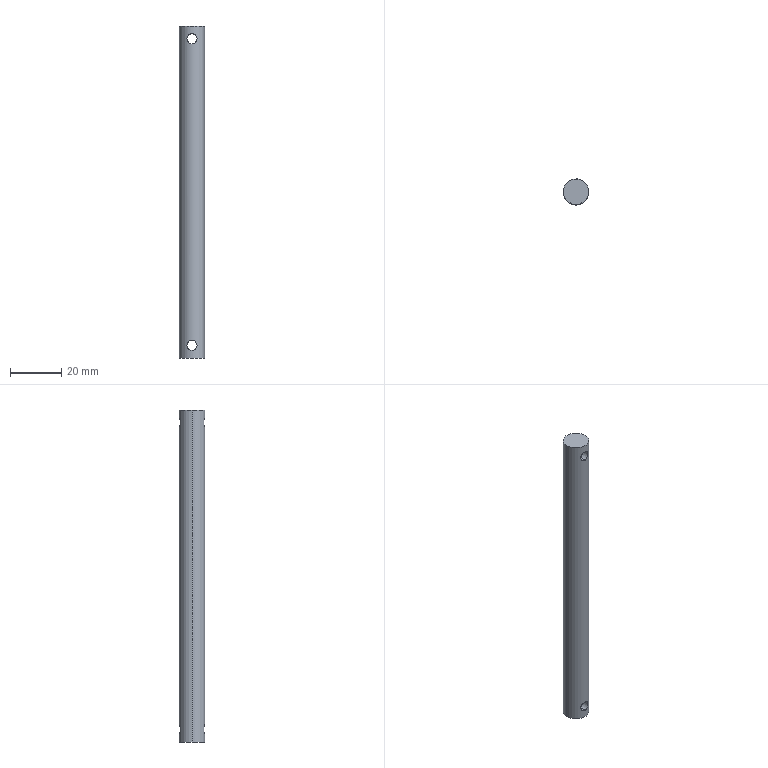Part | SolidWorks | features Extrusion 1, ICE 1 | 1 solid | 8 faces | box 10 x 10 x 130 mm | volume 9964 mm3 | cylinder 6 | plane 2 | commonest cylinder face diameters 4 x4 10 x2
STEP:
#1=CARTESIAN_POINT('',(0.,-5.,58.));
#2=VERTEX_POINT('',#1);
#3=CARTESIAN_POINT('',(0.,-5.,62.));
#4=VERTEX_POINT('',#3);
#5=CARTESIAN_POINT('',(0.,-5.,58.));
#6=CARTESIAN_POINT('',(-0.1316,-5.,58.));
#7=CARTESIAN_POINT('',(-0.2649,-4.995,58.013));
#8=CARTESIAN_POINT('',(-0.5241,-4.974,58.065));
#9=CARTESIAN_POINT('',(-0.6493,-4.959,58.104));
#10=CARTESIAN_POINT('',(-0.8912,-4.921,58.205));
#11=CARTESIAN_POINT('',(-1.008,-4.899,58.268));
#12=CARTESIAN_POINT('',(-1.223,-4.849,58.412));
#13=CARTESIAN_POINT('',(-1.323,-4.823,58.495));
#14=CARTESIAN_POINT('',(-1.507,-4.768,58.679));
#15=CARTESIAN_POINT('',(-1.589,-4.741,58.779));
#16=CARTESIAN_POINT('',(-1.733,-4.691,58.994));
#17=CARTESIAN_POINT('',(-1.796,-4.667,59.11));
#18=CARTESIAN_POINT('',(-1.896,-4.627,59.351));
#19=CARTESIAN_POINT('',(-1.935,-4.611,59.476));
#20=CARTESIAN_POINT('',(-1.987,-4.589,59.734));
#21=CARTESIAN_POINT('',(-2.,-4.583,59.868));
#22=CARTESIAN_POINT('',(-2.,-4.583,60.263));
#23=CARTESIAN_POINT('',(-1.946,-4.607,60.529));
#24=CARTESIAN_POINT('',(-1.796,-4.667,60.89));
#25=CARTESIAN_POINT('',(-1.733,-4.691,61.006));
#26=CARTESIAN_POINT('',(-1.589,-4.742,61.222));
#27=CARTESIAN_POINT('',(-1.507,-4.769,61.322));
#28=CARTESIAN_POINT('',(-1.323,-4.823,61.505));
#29=CARTESIAN_POINT('',(-1.222,-4.85,61.589));
#30=CARTESIAN_POINT('',(-1.007,-4.899,61.733));
#31=CARTESIAN_POINT('',(-0.8926,-4.921,61.795));
#32=CARTESIAN_POINT('',(-0.5273,-4.978,61.947));
#33=CARTESIAN_POINT('',(-0.2671,-5.,62.));
#34=CARTESIAN_POINT('',(0.,-5.,62.));
#35=B_SPLINE_CURVE_WITH_KNOTS('',3,(#5,#6,#7,#8,#9,#10,#11,#12,#13,#14,#15,#16,#17,#18,#19,#20,#21,#22,#23,#24,#25,#26,#27,#28,#29,#30,#31,#32,#33,#34),.UNSPECIFIED.,.F.,.F.,(4,2,2,2,2,2,2,2,2,2,2,2,2,2,4),(0.00632,0.006715,0.007109,0.007504,0.007899,0.008293,0.008688,0.009083,0.009478,0.01027,0.01066,0.01106,0.01145,0.01185,0.01264),.UNSPECIFIED.);
#36=EDGE_CURVE('',#2,#4,#35,.T.);
#37=ORIENTED_EDGE('',*,*,#36,.F.);
#38=CARTESIAN_POINT('',(0.,5.,58.));
#39=VERTEX_POINT('',#38);
#40=CARTESIAN_POINT('',(0.,-5.,58.));
#41=DIRECTION('',(0.,1.,0.));
#42=VECTOR('',#41,1000.);
#43=LINE('',#40,#42);
#44=EDGE_CURVE('',#2,#39,#43,.T.);
#45=ORIENTED_EDGE('',*,*,#44,.T.);
#46=CARTESIAN_POINT('',(0.,5.,62.));
#47=VERTEX_POINT('',#46);
#48=CARTESIAN_POINT('',(0.,5.,62.));
#49=CARTESIAN_POINT('',(-0.1337,5.,62.));
#50=CARTESIAN_POINT('',(-0.2648,4.995,61.987));
#51=CARTESIAN_POINT('',(-0.5224,4.974,61.935));
#52=CARTESIAN_POINT('',(-0.6502,4.959,61.896));
#53=CARTESIAN_POINT('',(-0.8919,4.921,61.795));
#54=CARTESIAN_POINT('',(-1.006,4.899,61.733));
#55=CARTESIAN_POINT('',(-1.223,4.849,61.588));
#56=CARTESIAN_POINT('',(-1.324,4.822,61.505));
#57=CARTESIAN_POINT('',(-1.597,4.742,61.231));
#58=CARTESIAN_POINT('',(-1.746,4.687,61.01));
#59=CARTESIAN_POINT('',(-1.896,4.627,60.65));
#60=CARTESIAN_POINT('',(-1.935,4.61,60.523));
#61=CARTESIAN_POINT('',(-1.987,4.588,60.264));
#62=CARTESIAN_POINT('',(-2.,4.583,60.133));
#63=CARTESIAN_POINT('',(-2.,4.583,59.869));
#64=CARTESIAN_POINT('',(-1.987,4.588,59.735));
#65=CARTESIAN_POINT('',(-1.935,4.611,59.477));
#66=CARTESIAN_POINT('',(-1.897,4.627,59.352));
#67=CARTESIAN_POINT('',(-1.795,4.667,59.108));
#68=CARTESIAN_POINT('',(-1.733,4.691,58.994));
#69=CARTESIAN_POINT('',(-1.589,4.741,58.778));
#70=CARTESIAN_POINT('',(-1.505,4.769,58.677));
#71=CARTESIAN_POINT('',(-1.322,4.823,58.494));
#72=CARTESIAN_POINT('',(-1.223,4.85,58.412));
#73=CARTESIAN_POINT('',(-1.006,4.899,58.267));
#74=CARTESIAN_POINT('',(-0.8898,4.922,58.204));
#75=CARTESIAN_POINT('',(-0.5291,4.978,58.054));
#76=CARTESIAN_POINT('',(-0.2633,5.,58.));
#77=CARTESIAN_POINT('',(0.,5.,58.));
#78=B_SPLINE_CURVE_WITH_KNOTS('',3,(#48,#49,#50,#51,#52,#53,#54,#55,#56,#57,#58,#59,#60,#61,#62,#63,#64,#65,#66,#67,#68,#69,#70,#71,#72,#73,#74,#75,#76,#77),.UNSPECIFIED.,.F.,.F.,(4,2,2,2,2,2,2,2,2,2,2,2,2,2,4),(0.,0.000395,0.00079,0.001185,0.00158,0.00237,0.002765,0.00316,0.003555,0.00395,0.004345,0.00474,0.005135,0.00553,0.00632),.UNSPECIFIED.);
#79=EDGE_CURVE('',#47,#39,#78,.T.);
#80=ORIENTED_EDGE('',*,*,#79,.F.);
#81=CARTESIAN_POINT('',(0.,-5.,62.));
#82=DIRECTION('',(0.,1.,0.));
#83=VECTOR('',#82,1000.);
#84=LINE('',#81,#83);
#85=EDGE_CURVE('',#4,#47,#84,.T.);
#86=ORIENTED_EDGE('',*,*,#85,.F.);
#87=EDGE_LOOP('',(#37,#45,#80,#86));
#88=FACE_OUTER_BOUND('',#87,.T.);
#89=CARTESIAN_POINT('',(0.,-5.,60.));
#90=DIRECTION('',(0.,1.,0.));
#91=DIRECTION('',(0.,0.,1.));
#92=AXIS2_PLACEMENT_3D('',#89,#90,#91);
#93=CYLINDRICAL_SURFACE('',#92,2.);
#94=ADVANCED_FACE('',(#88),#93,.F.);
#95=CARTESIAN_POINT('',(0.,-5.,-62.));
#96=VERTEX_POINT('',#95);
#97=CARTESIAN_POINT('',(0.,-5.,-58.));
#98=VERTEX_POINT('',#97);
#99=CARTESIAN_POINT('',(0.,-5.,-62.));
#100=CARTESIAN_POINT('',(-0.1316,-5.,-62.));
#101=CARTESIAN_POINT('',(-0.2649,-4.995,-61.987));
#102=CARTESIAN_POINT('',(-0.5241,-4.974,-61.935));
#103=CARTESIAN_POINT('',(-0.6493,-4.959,-61.896));
#104=CARTESIAN_POINT('',(-0.8912,-4.921,-61.795));
#105=CARTESIAN_POINT('',(-1.008,-4.899,-61.732));
#106=CARTESIAN_POINT('',(-1.223,-4.849,-61.588));
#107=CARTESIAN_POINT('',(-1.323,-4.823,-61.505));
#108=CARTESIAN_POINT('',(-1.507,-4.768,-61.321));
#109=CARTESIAN_POINT('',(-1.589,-4.741,-61.221));
#110=CARTESIAN_POINT('',(-1.733,-4.691,-61.006));
#111=CARTESIAN_POINT('',(-1.796,-4.667,-60.89));
#112=CARTESIAN_POINT('',(-1.896,-4.627,-60.649));
#113=CARTESIAN_POINT('',(-1.935,-4.611,-60.524));
#114=CARTESIAN_POINT('',(-1.987,-4.589,-60.266));
#115=CARTESIAN_POINT('',(-2.,-4.583,-60.132));
#116=CARTESIAN_POINT('',(-2.,-4.583,-59.737));
#117=CARTESIAN_POINT('',(-1.946,-4.607,-59.471));
#118=CARTESIAN_POINT('',(-1.796,-4.667,-59.11));
#119=CARTESIAN_POINT('',(-1.733,-4.691,-58.994));
#120=CARTESIAN_POINT('',(-1.589,-4.742,-58.778));
#121=CARTESIAN_POINT('',(-1.507,-4.769,-58.678));
#122=CARTESIAN_POINT('',(-1.323,-4.823,-58.495));
#123=CARTESIAN_POINT('',(-1.222,-4.85,-58.411));
#124=CARTESIAN_POINT('',(-1.007,-4.899,-58.267));
#125=CARTESIAN_POINT('',(-0.8926,-4.921,-58.205));
#126=CARTESIAN_POINT('',(-0.5273,-4.978,-58.053));
#127=CARTESIAN_POINT('',(-0.2671,-5.,-58.));
#128=CARTESIAN_POINT('',(0.,-5.,-58.));
#129=B_SPLINE_CURVE_WITH_KNOTS('',3,(#99,#100,#101,#102,#103,#104,#105,#106,#107,#108,#109,#110,#111,#112,#113,#114,#115,#116,#117,#118,#119,#120,#121,#122,#123,#124,#125,#126,#127,#128),.UNSPECIFIED.,.F.,.F.,(4,2,2,2,2,2,2,2,2,2,2,2,2,2,4),(0.00632,0.006715,0.007109,0.007504,0.007899,0.008293,0.008688,0.009083,0.009478,0.01027,0.01066,0.01106,0.01145,0.01185,0.01264),.UNSPECIFIED.);
#130=EDGE_CURVE('',#96,#98,#129,.T.);
#131=ORIENTED_EDGE('',*,*,#130,.F.);
#132=CARTESIAN_POINT('',(0.,5.,-62.));
#133=VERTEX_POINT('',#132);
#134=CARTESIAN_POINT('',(0.,-5.,-62.));
#135=DIRECTION('',(0.,1.,0.));
#136=VECTOR('',#135,1000.);
#137=LINE('',#134,#136);
#138=EDGE_CURVE('',#96,#133,#137,.T.);
#139=ORIENTED_EDGE('',*,*,#138,.T.);
#140=CARTESIAN_POINT('',(0.,5.,-58.));
#141=VERTEX_POINT('',#140);
#142=CARTESIAN_POINT('',(0.,5.,-58.));
#143=CARTESIAN_POINT('',(-0.1337,5.,-58.));
#144=CARTESIAN_POINT('',(-0.2648,4.995,-58.013));
#145=CARTESIAN_POINT('',(-0.5224,4.974,-58.065));
#146=CARTESIAN_POINT('',(-0.6502,4.959,-58.104));
#147=CARTESIAN_POINT('',(-0.8919,4.921,-58.205));
#148=CARTESIAN_POINT('',(-1.006,4.899,-58.267));
#149=CARTESIAN_POINT('',(-1.223,4.849,-58.412));
#150=CARTESIAN_POINT('',(-1.324,4.822,-58.495));
#151=CARTESIAN_POINT('',(-1.597,4.742,-58.769));
#152=CARTESIAN_POINT('',(-1.746,4.687,-58.99));
#153=CARTESIAN_POINT('',(-1.896,4.627,-59.35));
#154=CARTESIAN_POINT('',(-1.935,4.61,-59.477));
#155=CARTESIAN_POINT('',(-1.987,4.588,-59.736));
#156=CARTESIAN_POINT('',(-2.,4.583,-59.867));
#157=CARTESIAN_POINT('',(-2.,4.583,-60.131));
#158=CARTESIAN_POINT('',(-1.987,4.588,-60.265));
#159=CARTESIAN_POINT('',(-1.935,4.611,-60.523));
#160=CARTESIAN_POINT('',(-1.897,4.627,-60.648));
#161=CARTESIAN_POINT('',(-1.795,4.667,-60.892));
#162=CARTESIAN_POINT('',(-1.733,4.691,-61.006));
#163=CARTESIAN_POINT('',(-1.589,4.741,-61.222));
#164=CARTESIAN_POINT('',(-1.505,4.769,-61.323));
#165=CARTESIAN_POINT('',(-1.322,4.823,-61.506));
#166=CARTESIAN_POINT('',(-1.223,4.85,-61.588));
#167=CARTESIAN_POINT('',(-1.006,4.899,-61.733));
#168=CARTESIAN_POINT('',(-0.8898,4.922,-61.796));
#169=CARTESIAN_POINT('',(-0.5291,4.978,-61.946));
#170=CARTESIAN_POINT('',(-0.2633,5.,-62.));
#171=CARTESIAN_POINT('',(0.,5.,-62.));
#172=B_SPLINE_CURVE_WITH_KNOTS('',3,(#142,#143,#144,#145,#146,#147,#148,#149,#150,#151,#152,#153,#154,#155,#156,#157,#158,#159,#160,#161,#162,#163,#164,#165,#166,#167,#168,#169,#170,#171),.UNSPECIFIED.,.F.,.F.,(4,2,2,2,2,2,2,2,2,2,2,2,2,2,4),(0.,0.000395,0.00079,0.001185,0.00158,0.00237,0.002765,0.00316,0.003555,0.00395,0.004345,0.00474,0.005135,0.00553,0.00632),.UNSPECIFIED.);
#173=EDGE_CURVE('',#141,#133,#172,.T.);
#174=ORIENTED_EDGE('',*,*,#173,.F.);
#175=CARTESIAN_POINT('',(0.,-5.,-58.));
#176=DIRECTION('',(0.,1.,0.));
#177=VECTOR('',#176,1000.);
#178=LINE('',#175,#177);
#179=EDGE_CURVE('',#98,#141,#178,.T.);
#180=ORIENTED_EDGE('',*,*,#179,.F.);
#181=EDGE_LOOP('',(#131,#139,#174,#180));
#182=FACE_OUTER_BOUND('',#181,.T.);
#183=CARTESIAN_POINT('',(0.,-5.,-60.));
#184=DIRECTION('',(0.,1.,0.));
#185=DIRECTION('',(0.,0.,1.));
#186=AXIS2_PLACEMENT_3D('',#183,#184,#185);
#187=CYLINDRICAL_SURFACE('',#186,2.);
#188=ADVANCED_FACE('',(#182),#187,.F.);
#189=ORIENTED_EDGE('',*,*,#173,.T.);
#190=CARTESIAN_POINT('',(0.,5.,-62.));
#191=CARTESIAN_POINT('',(0.1316,5.,-62.));
#192=CARTESIAN_POINT('',(0.2649,4.995,-61.987));
#193=CARTESIAN_POINT('',(0.5241,4.974,-61.935));
#194=CARTESIAN_POINT('',(0.6493,4.959,-61.896));
#195=CARTESIAN_POINT('',(0.8912,4.921,-61.795));
#196=CARTESIAN_POINT('',(1.008,4.899,-61.732));
#197=CARTESIAN_POINT('',(1.223,4.849,-61.588));
#198=CARTESIAN_POINT('',(1.323,4.823,-61.505));
#199=CARTESIAN_POINT('',(1.507,4.768,-61.321));
#200=CARTESIAN_POINT('',(1.589,4.741,-61.221));
#201=CARTESIAN_POINT('',(1.733,4.691,-61.006));
#202=CARTESIAN_POINT('',(1.796,4.667,-60.89));
#203=CARTESIAN_POINT('',(1.896,4.627,-60.649));
#204=CARTESIAN_POINT('',(1.935,4.611,-60.524));
#205=CARTESIAN_POINT('',(1.987,4.589,-60.266));
#206=CARTESIAN_POINT('',(2.,4.583,-60.132));
#207=CARTESIAN_POINT('',(2.,4.583,-59.737));
#208=CARTESIAN_POINT('',(1.946,4.607,-59.471));
#209=CARTESIAN_POINT('',(1.796,4.667,-59.11));
#210=CARTESIAN_POINT('',(1.733,4.691,-58.994));
#211=CARTESIAN_POINT('',(1.589,4.742,-58.778));
#212=CARTESIAN_POINT('',(1.507,4.769,-58.678));
#213=CARTESIAN_POINT('',(1.323,4.823,-58.495));
#214=CARTESIAN_POINT('',(1.222,4.85,-58.411));
#215=CARTESIAN_POINT('',(1.007,4.899,-58.267));
#216=CARTESIAN_POINT('',(0.8926,4.921,-58.205));
#217=CARTESIAN_POINT('',(0.5273,4.978,-58.053));
#218=CARTESIAN_POINT('',(0.2671,5.,-58.));
#219=CARTESIAN_POINT('',(0.,5.,-58.));
#220=B_SPLINE_CURVE_WITH_KNOTS('',3,(#190,#191,#192,#193,#194,#195,#196,#197,#198,#199,#200,#201,#202,#203,#204,#205,#206,#207,#208,#209,#210,#211,#212,#213,#214,#215,#216,#217,#218,#219),.UNSPECIFIED.,.F.,.F.,(4,2,2,2,2,2,2,2,2,2,2,2,2,2,4),(0.00632,0.006715,0.007109,0.007504,0.007899,0.008293,0.008688,0.009083,0.009478,0.01027,0.01066,0.01106,0.01145,0.01185,0.01264),.UNSPECIFIED.);
#221=EDGE_CURVE('',#133,#141,#220,.T.);
#222=ORIENTED_EDGE('',*,*,#221,.T.);
#223=EDGE_LOOP('',(#189,#222));
#224=FACE_BOUND('',#223,.T.);
#225=ORIENTED_EDGE('',*,*,#79,.T.);
#226=CARTESIAN_POINT('',(0.,5.,58.));
#227=CARTESIAN_POINT('',(0.1316,5.,58.));
#228=CARTESIAN_POINT('',(0.2649,4.995,58.013));
#229=CARTESIAN_POINT('',(0.5241,4.974,58.065));
#230=CARTESIAN_POINT('',(0.6493,4.959,58.104));
#231=CARTESIAN_POINT('',(0.8912,4.921,58.205));
#232=CARTESIAN_POINT('',(1.008,4.899,58.268));
#233=CARTESIAN_POINT('',(1.223,4.849,58.412));
#234=CARTESIAN_POINT('',(1.323,4.823,58.495));
#235=CARTESIAN_POINT('',(1.507,4.768,58.679));
#236=CARTESIAN_POINT('',(1.589,4.741,58.779));
#237=CARTESIAN_POINT('',(1.733,4.691,58.994));
#238=CARTESIAN_POINT('',(1.796,4.667,59.11));
#239=CARTESIAN_POINT('',(1.896,4.627,59.351));
#240=CARTESIAN_POINT('',(1.935,4.611,59.476));
#241=CARTESIAN_POINT('',(1.987,4.589,59.734));
#242=CARTESIAN_POINT('',(2.,4.583,59.868));
#243=CARTESIAN_POINT('',(2.,4.583,60.263));
#244=CARTESIAN_POINT('',(1.946,4.607,60.529));
#245=CARTESIAN_POINT('',(1.796,4.667,60.89));
#246=CARTESIAN_POINT('',(1.733,4.691,61.006));
#247=CARTESIAN_POINT('',(1.589,4.742,61.222));
#248=CARTESIAN_POINT('',(1.507,4.769,61.322));
#249=CARTESIAN_POINT('',(1.323,4.823,61.505));
#250=CARTESIAN_POINT('',(1.222,4.85,61.589));
#251=CARTESIAN_POINT('',(1.007,4.899,61.733));
#252=CARTESIAN_POINT('',(0.8926,4.921,61.795));
#253=CARTESIAN_POINT('',(0.5273,4.978,61.947));
#254=CARTESIAN_POINT('',(0.2671,5.,62.));
#255=CARTESIAN_POINT('',(0.,5.,62.));
#256=B_SPLINE_CURVE_WITH_KNOTS('',3,(#226,#227,#228,#229,#230,#231,#232,#233,#234,#235,#236,#237,#238,#239,#240,#241,#242,#243,#244,#245,#246,#247,#248,#249,#250,#251,#252,#253,#254,#255),.UNSPECIFIED.,.F.,.F.,(4,2,2,2,2,2,2,2,2,2,2,2,2,2,4),(0.00632,0.006715,0.007109,0.007504,0.007899,0.008293,0.008688,0.009083,0.009478,0.01027,0.01066,0.01106,0.01145,0.01185,0.01264),.UNSPECIFIED.);
#257=EDGE_CURVE('',#39,#47,#256,.T.);
#258=ORIENTED_EDGE('',*,*,#257,.T.);
#259=EDGE_LOOP('',(#225,#258));
#260=FACE_BOUND('',#259,.T.);
#261=CARTESIAN_POINT('',(5.,0.,65.));
#262=VERTEX_POINT('',#261);
#263=CARTESIAN_POINT('',(-5.,0.,65.));
#264=VERTEX_POINT('',#263);
#265=CARTESIAN_POINT('',(0.,0.,65.));
#266=DIRECTION('',(0.,0.,1.));
#267=DIRECTION('',(1.,0.,0.));
#268=AXIS2_PLACEMENT_3D('',#265,#266,#267);
#269=CIRCLE('',#268,5.);
#270=EDGE_CURVE('',#262,#264,#269,.T.);
#271=ORIENTED_EDGE('',*,*,#270,.F.);
#272=CARTESIAN_POINT('',(5.,0.,-65.));
#273=VERTEX_POINT('',#272);
#274=CARTESIAN_POINT('',(5.,0.,65.));
#275=DIRECTION('',(0.,0.,-1.));
#276=VECTOR('',#275,1000.);
#277=LINE('',#274,#276);
#278=EDGE_CURVE('',#262,#273,#277,.T.);
#279=ORIENTED_EDGE('',*,*,#278,.T.);
#280=CARTESIAN_POINT('',(-5.,0.,-65.));
#281=VERTEX_POINT('',#280);
#282=CARTESIAN_POINT('',(0.,0.,-65.));
#283=DIRECTION('',(0.,0.,1.));
#284=DIRECTION('',(1.,0.,0.));
#285=AXIS2_PLACEMENT_3D('',#282,#283,#284);
#286=CIRCLE('',#285,5.);
#287=EDGE_CURVE('',#273,#281,#286,.T.);
#288=ORIENTED_EDGE('',*,*,#287,.T.);
#289=CARTESIAN_POINT('',(-5.,0.,65.));
#290=DIRECTION('',(0.,0.,-1.));
#291=VECTOR('',#290,1000.);
#292=LINE('',#289,#291);
#293=EDGE_CURVE('',#264,#281,#292,.T.);
#294=ORIENTED_EDGE('',*,*,#293,.F.);
#295=EDGE_LOOP('',(#271,#279,#288,#294));
#296=FACE_OUTER_BOUND('',#295,.T.);
#297=CARTESIAN_POINT('',(0.,0.,65.));
#298=DIRECTION('',(0.,0.,-1.));
#299=DIRECTION('',(-1.,0.,0.));
#300=AXIS2_PLACEMENT_3D('',#297,#298,#299);
#301=CYLINDRICAL_SURFACE('',#300,5.);
#302=ADVANCED_FACE('',(#224,#260,#296),#301,.T.);
#303=ORIENTED_EDGE('',*,*,#278,.F.);
#304=CARTESIAN_POINT('',(0.,0.,65.));
#305=DIRECTION('',(0.,0.,1.));
#306=DIRECTION('',(1.,0.,0.));
#307=AXIS2_PLACEMENT_3D('',#304,#305,#306);
#308=CIRCLE('',#307,5.);
#309=EDGE_CURVE('',#264,#262,#308,.T.);
#310=ORIENTED_EDGE('',*,*,#309,.F.);
#311=ORIENTED_EDGE('',*,*,#293,.T.);
#312=CARTESIAN_POINT('',(0.,0.,-65.));
#313=DIRECTION('',(0.,0.,1.));
#314=DIRECTION('',(1.,0.,0.));
#315=AXIS2_PLACEMENT_3D('',#312,#313,#314);
#316=CIRCLE('',#315,5.);
#317=EDGE_CURVE('',#281,#273,#316,.T.);
#318=ORIENTED_EDGE('',*,*,#317,.T.);
#319=EDGE_LOOP('',(#303,#310,#311,#318));
#320=FACE_OUTER_BOUND('',#319,.T.);
#321=CARTESIAN_POINT('',(0.,-5.,62.));
#322=CARTESIAN_POINT('',(0.1337,-5.,62.));
#323=CARTESIAN_POINT('',(0.2648,-4.995,61.987));
#324=CARTESIAN_POINT('',(0.5224,-4.974,61.935));
#325=CARTESIAN_POINT('',(0.6502,-4.959,61.896));
#326=CARTESIAN_POINT('',(0.8919,-4.921,61.795));
#327=CARTESIAN_POINT('',(1.006,-4.899,61.733));
#328=CARTESIAN_POINT('',(1.223,-4.849,61.588));
#329=CARTESIAN_POINT('',(1.324,-4.822,61.505));
#330=CARTESIAN_POINT('',(1.597,-4.742,61.231));
#331=CARTESIAN_POINT('',(1.746,-4.687,61.01));
#332=CARTESIAN_POINT('',(1.896,-4.627,60.65));
#333=CARTESIAN_POINT('',(1.935,-4.61,60.523));
#334=CARTESIAN_POINT('',(1.987,-4.588,60.264));
#335=CARTESIAN_POINT('',(2.,-4.583,60.133));
#336=CARTESIAN_POINT('',(2.,-4.583,59.869));
#337=CARTESIAN_POINT('',(1.987,-4.588,59.735));
#338=CARTESIAN_POINT('',(1.935,-4.611,59.477));
#339=CARTESIAN_POINT('',(1.897,-4.627,59.352));
#340=CARTESIAN_POINT('',(1.795,-4.667,59.108));
#341=CARTESIAN_POINT('',(1.733,-4.691,58.994));
#342=CARTESIAN_POINT('',(1.589,-4.741,58.778));
#343=CARTESIAN_POINT('',(1.505,-4.769,58.677));
#344=CARTESIAN_POINT('',(1.322,-4.823,58.494));
#345=CARTESIAN_POINT('',(1.223,-4.85,58.412));
#346=CARTESIAN_POINT('',(1.006,-4.899,58.267));
#347=CARTESIAN_POINT('',(0.8898,-4.922,58.204));
#348=CARTESIAN_POINT('',(0.5291,-4.978,58.054));
#349=CARTESIAN_POINT('',(0.2633,-5.,58.));
#350=CARTESIAN_POINT('',(0.,-5.,58.));
#351=B_SPLINE_CURVE_WITH_KNOTS('',3,(#321,#322,#323,#324,#325,#326,#327,#328,#329,#330,#331,#332,#333,#334,#335,#336,#337,#338,#339,#340,#341,#342,#343,#344,#345,#346,#347,#348,#349,#350),.UNSPECIFIED.,.F.,.F.,(4,2,2,2,2,2,2,2,2,2,2,2,2,2,4),(0.,0.000395,0.00079,0.001185,0.00158,0.00237,0.002765,0.00316,0.003555,0.00395,0.004345,0.00474,0.005135,0.00553,0.00632),.UNSPECIFIED.);
#352=EDGE_CURVE('',#4,#2,#351,.T.);
#353=ORIENTED_EDGE('',*,*,#352,.T.);
#354=ORIENTED_EDGE('',*,*,#36,.T.);
#355=EDGE_LOOP('',(#353,#354));
#356=FACE_BOUND('',#355,.T.);
#357=CARTESIAN_POINT('',(0.,-5.,-58.));
#358=CARTESIAN_POINT('',(0.1337,-5.,-58.));
#359=CARTESIAN_POINT('',(0.2648,-4.995,-58.013));
#360=CARTESIAN_POINT('',(0.5224,-4.974,-58.065));
#361=CARTESIAN_POINT('',(0.6502,-4.959,-58.104));
#362=CARTESIAN_POINT('',(0.8919,-4.921,-58.205));
#363=CARTESIAN_POINT('',(1.006,-4.899,-58.267));
#364=CARTESIAN_POINT('',(1.223,-4.849,-58.412));
#365=CARTESIAN_POINT('',(1.324,-4.822,-58.495));
#366=CARTESIAN_POINT('',(1.597,-4.742,-58.769));
#367=CARTESIAN_POINT('',(1.746,-4.687,-58.99));
#368=CARTESIAN_POINT('',(1.896,-4.627,-59.35));
#369=CARTESIAN_POINT('',(1.935,-4.61,-59.477));
#370=CARTESIAN_POINT('',(1.987,-4.588,-59.736));
#371=CARTESIAN_POINT('',(2.,-4.583,-59.867));
#372=CARTESIAN_POINT('',(2.,-4.583,-60.131));
#373=CARTESIAN_POINT('',(1.987,-4.588,-60.265));
#374=CARTESIAN_POINT('',(1.935,-4.611,-60.523));
#375=CARTESIAN_POINT('',(1.897,-4.627,-60.648));
#376=CARTESIAN_POINT('',(1.795,-4.667,-60.892));
#377=CARTESIAN_POINT('',(1.733,-4.691,-61.006));
#378=CARTESIAN_POINT('',(1.589,-4.741,-61.222));
#379=CARTESIAN_POINT('',(1.505,-4.769,-61.323));
#380=CARTESIAN_POINT('',(1.322,-4.823,-61.506));
#381=CARTESIAN_POINT('',(1.223,-4.85,-61.588));
#382=CARTESIAN_POINT('',(1.006,-4.899,-61.733));
#383=CARTESIAN_POINT('',(0.8898,-4.922,-61.796));
#384=CARTESIAN_POINT('',(0.5291,-4.978,-61.946));
#385=CARTESIAN_POINT('',(0.2633,-5.,-62.));
#386=CARTESIAN_POINT('',(0.,-5.,-62.));
#387=B_SPLINE_CURVE_WITH_KNOTS('',3,(#357,#358,#359,#360,#361,#362,#363,#364,#365,#366,#367,#368,#369,#370,#371,#372,#373,#374,#375,#376,#377,#378,#379,#380,#381,#382,#383,#384,#385,#386),.UNSPECIFIED.,.F.,.F.,(4,2,2,2,2,2,2,2,2,2,2,2,2,2,4),(0.,0.000395,0.00079,0.001185,0.00158,0.00237,0.002765,0.00316,0.003555,0.00395,0.004345,0.00474,0.005135,0.00553,0.00632),.UNSPECIFIED.);
#388=EDGE_CURVE('',#98,#96,#387,.T.);
#389=ORIENTED_EDGE('',*,*,#388,.T.);
#390=ORIENTED_EDGE('',*,*,#130,.T.);
#391=EDGE_LOOP('',(#389,#390));
#392=FACE_BOUND('',#391,.T.);
#393=CARTESIAN_POINT('',(0.,0.,65.));
#394=DIRECTION('',(0.,0.,-1.));
#395=DIRECTION('',(-1.,0.,0.));
#396=AXIS2_PLACEMENT_3D('',#393,#394,#395);
#397=CYLINDRICAL_SURFACE('',#396,5.);
#398=ADVANCED_FACE('',(#320,#356,#392),#397,.T.);
#399=ORIENTED_EDGE('',*,*,#309,.T.);
#400=ORIENTED_EDGE('',*,*,#270,.T.);
#401=EDGE_LOOP('',(#399,#400));
#402=FACE_OUTER_BOUND('',#401,.T.);
#403=CARTESIAN_POINT('',(0.,0.,65.));
#404=DIRECTION('',(0.,0.,1.));
#405=DIRECTION('',(1.,0.,0.));
#406=AXIS2_PLACEMENT_3D('',#403,#404,#405);
#407=PLANE('',#406);
#408=ADVANCED_FACE('',(#402),#407,.T.);
#409=ORIENTED_EDGE('',*,*,#317,.F.);
#410=ORIENTED_EDGE('',*,*,#287,.F.);
#411=EDGE_LOOP('',(#409,#410));
#412=FACE_OUTER_BOUND('',#411,.T.);
#413=CARTESIAN_POINT('',(0.,0.,-65.));
#414=DIRECTION('',(0.,0.,1.));
#415=DIRECTION('',(1.,0.,0.));
#416=AXIS2_PLACEMENT_3D('',#413,#414,#415);
#417=PLANE('',#416);
#418=ADVANCED_FACE('',(#412),#417,.F.);
#419=ORIENTED_EDGE('',*,*,#138,.F.);
#420=ORIENTED_EDGE('',*,*,#388,.F.);
#421=ORIENTED_EDGE('',*,*,#179,.T.);
#422=ORIENTED_EDGE('',*,*,#221,.F.);
#423=EDGE_LOOP('',(#419,#420,#421,#422));
#424=FACE_OUTER_BOUND('',#423,.T.);
#425=CARTESIAN_POINT('',(0.,-5.,-60.));
#426=DIRECTION('',(0.,1.,0.));
#427=DIRECTION('',(0.,0.,1.));
#428=AXIS2_PLACEMENT_3D('',#425,#426,#427);
#429=CYLINDRICAL_SURFACE('',#428,2.);
#430=ADVANCED_FACE('',(#424),#429,.F.);
#431=ORIENTED_EDGE('',*,*,#44,.F.);
#432=ORIENTED_EDGE('',*,*,#352,.F.);
#433=ORIENTED_EDGE('',*,*,#85,.T.);
#434=ORIENTED_EDGE('',*,*,#257,.F.);
#435=EDGE_LOOP('',(#431,#432,#433,#434));
#436=FACE_OUTER_BOUND('',#435,.T.);
#437=CARTESIAN_POINT('',(0.,-5.,60.));
#438=DIRECTION('',(0.,1.,0.));
#439=DIRECTION('',(0.,0.,1.));
#440=AXIS2_PLACEMENT_3D('',#437,#438,#439);
#441=CYLINDRICAL_SURFACE('',#440,2.);
#442=ADVANCED_FACE('',(#436),#441,.F.);
#443=CLOSED_SHELL('',(#94,#188,#302,#398,#408,#418,#430,#442));
#444=MANIFOLD_SOLID_BREP('',#443);
#445=CARTESIAN_POINT('',(0.,0.,0.));
#446=DIRECTION('',(0.,0.,1.));
#447=DIRECTION('',(1.,0.,0.));
#448=AXIS2_PLACEMENT_3D('',#445,#446,#447);
#449=(LENGTH_UNIT()NAMED_UNIT(*)SI_UNIT(.MILLI.,.METRE.));
#450=UNCERTAINTY_MEASURE_WITH_UNIT(LENGTH_MEASURE(0.00001),#449,'','');
#451=(NAMED_UNIT(*)PLANE_ANGLE_UNIT()SI_UNIT($,.RADIAN.));
#452=(NAMED_UNIT(*)SI_UNIT($,.STERADIAN.)SOLID_ANGLE_UNIT());
#453=(GEOMETRIC_REPRESENTATION_CONTEXT(3)GLOBAL_UNCERTAINTY_ASSIGNED_CONTEXT((#450))GLOBAL_UNIT_ASSIGNED_CONTEXT((#449,#451,#452))REPRESENTATION_CONTEXT('',''));
#454=ADVANCED_BREP_SHAPE_REPRESENTATION('',(#444,#448),#453);